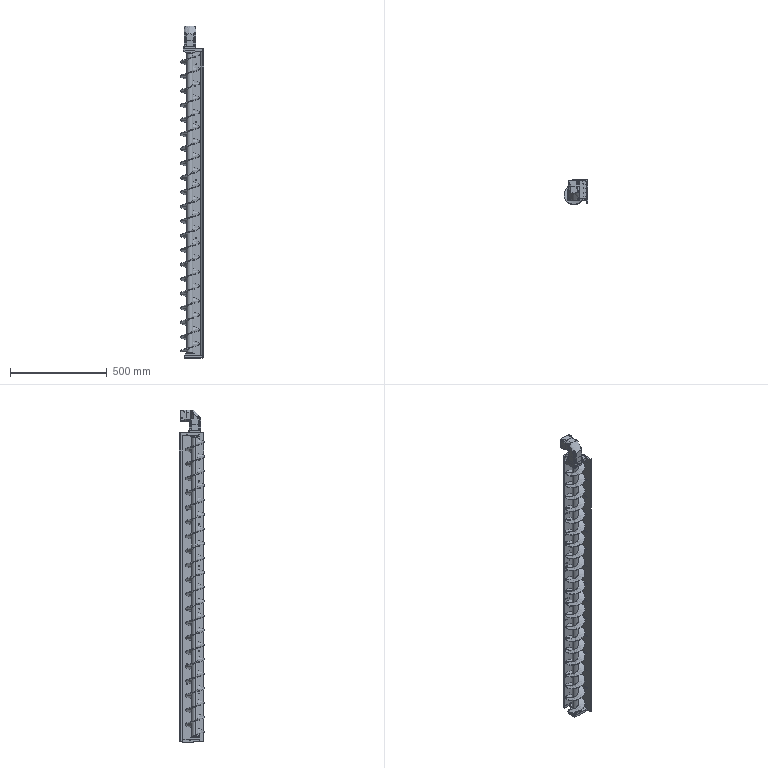Part | SolidWorks | 21 solids | 1030 faces | box 122 x 130 x 1720 mm | volume 4058025 mm3 | cylinder 550 | plane 296 | cone 111 | spline 53 | torus 20 | commonest cylinder face diameters 4.2 x190 5.5 x40 10.1 x30 10 x28 69 x26 3.3 x18